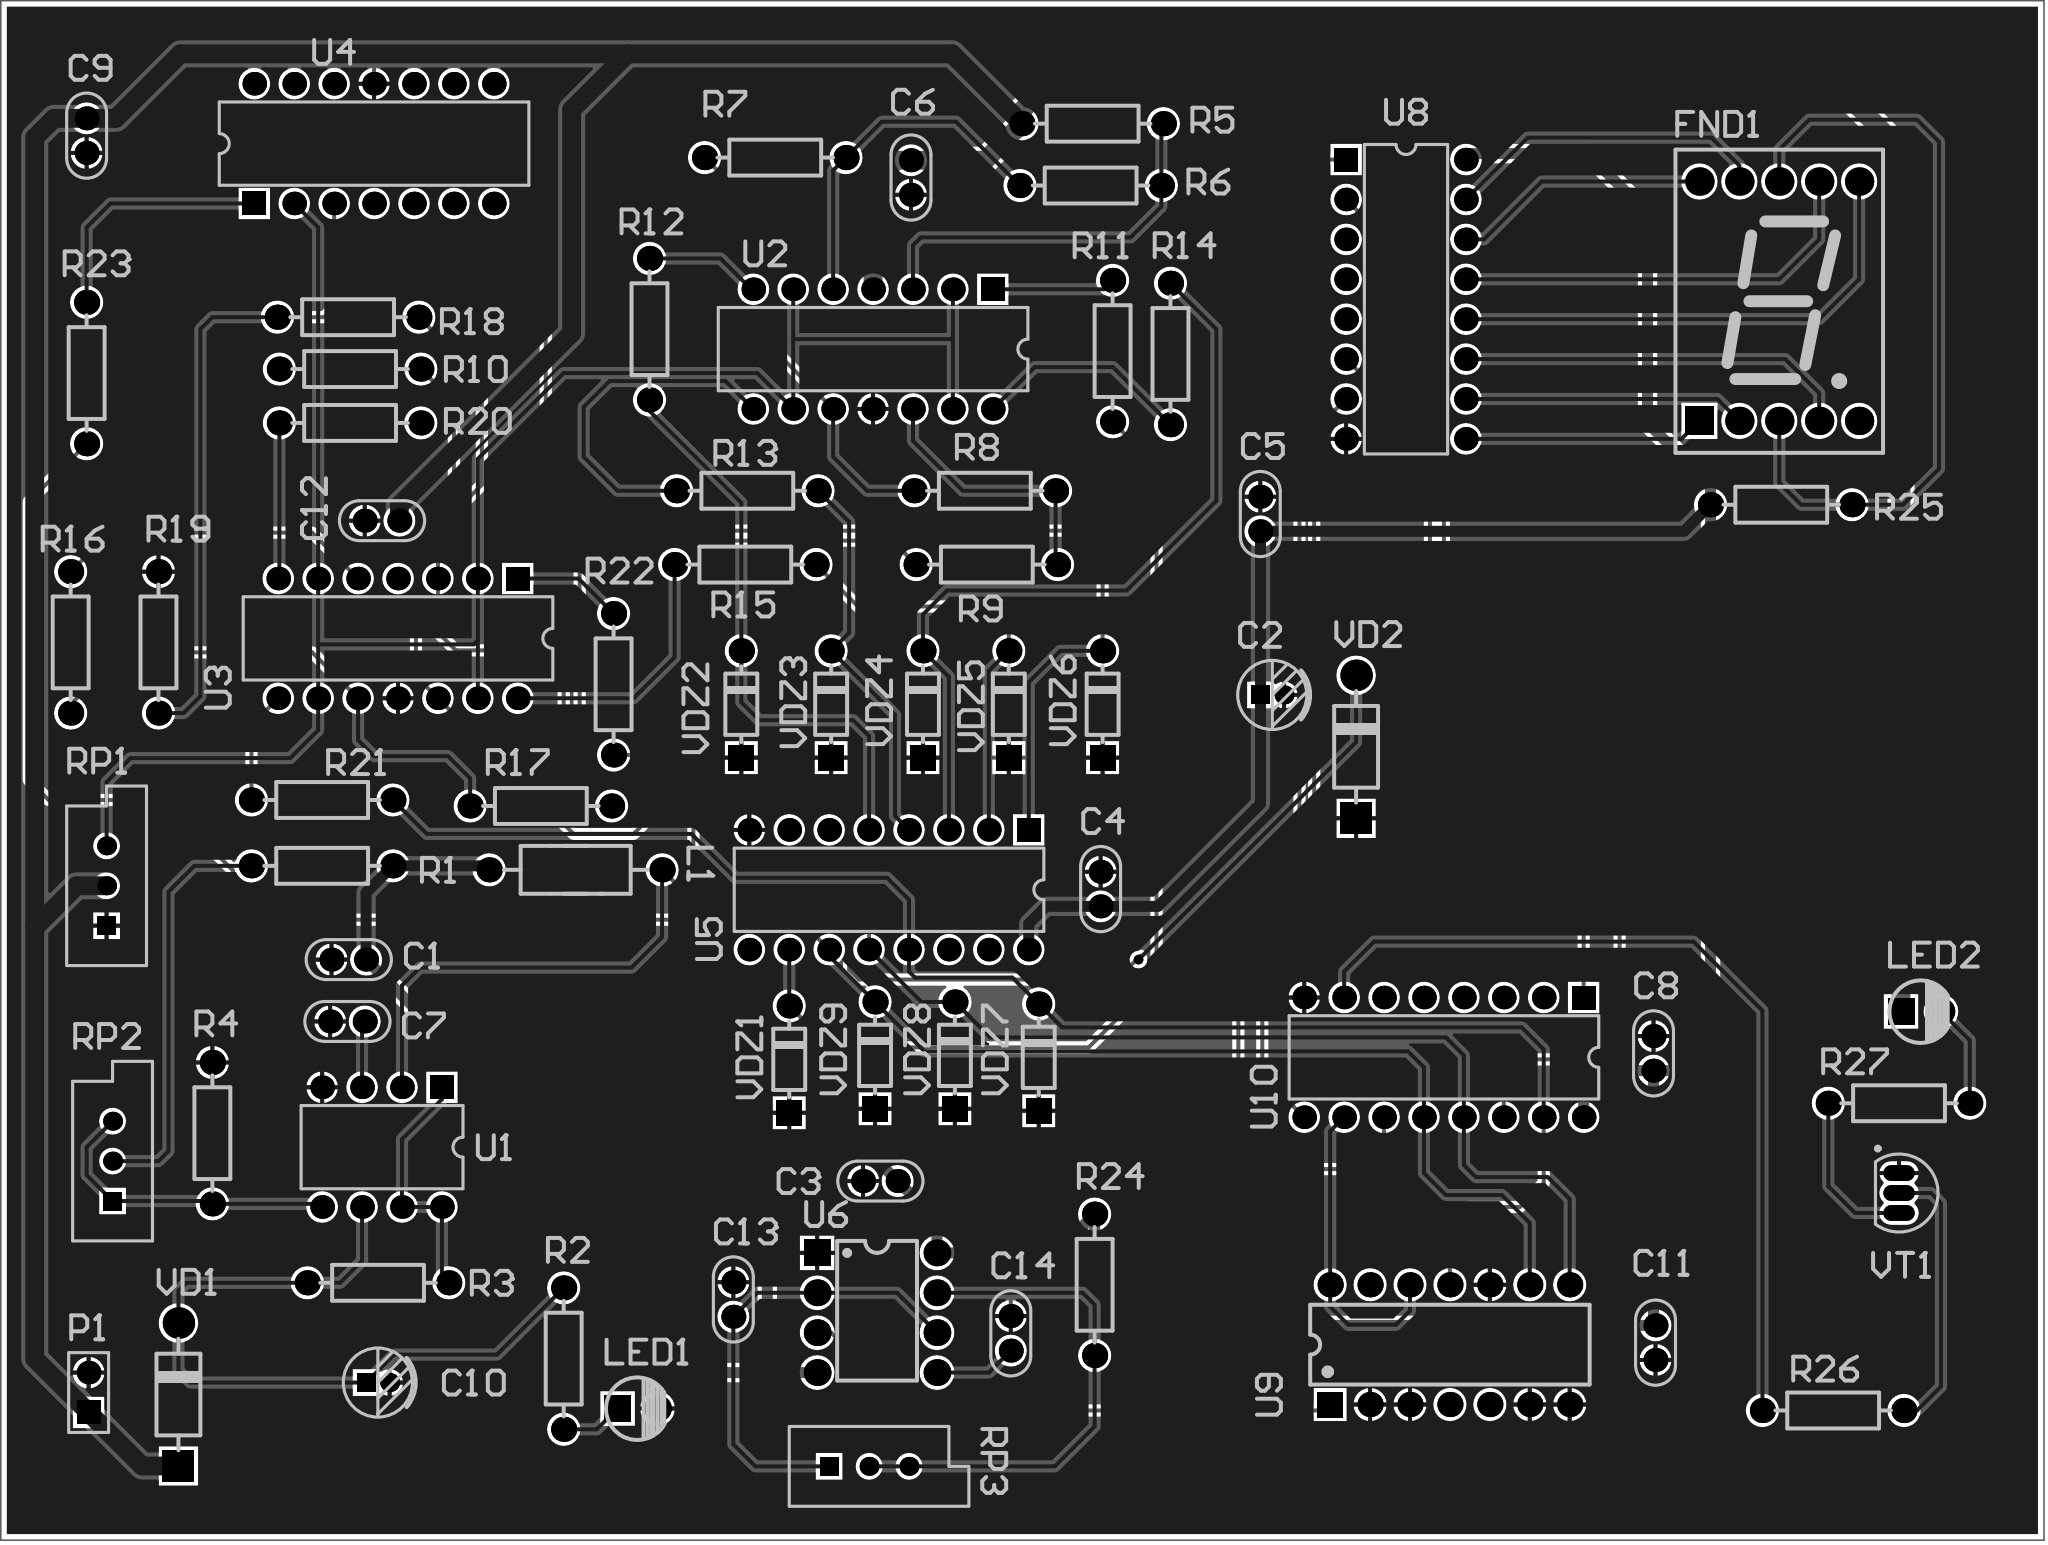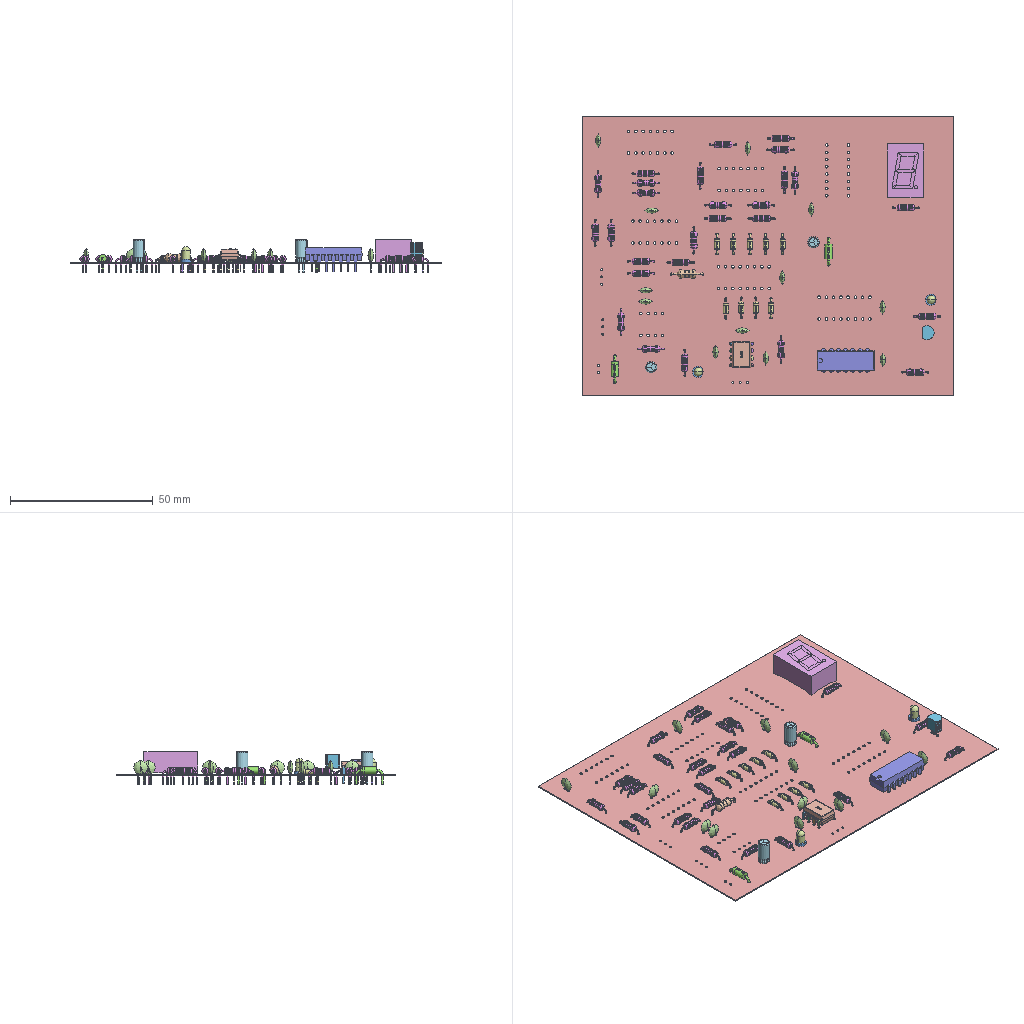Circuit board layout | Altium Designer | box 130 x 98 x 11.6 mm
Layer stack:
# Altium Designer layer stack of  (unit mm; dielectric type: 0 none, 1 core, 2 prepreg, 3 surface material)
index,name,kind,layer,copper_thickness_mm,dielectric_type,dielectric_thickness_mm,dielectric_material,dielectric_constant
0,Top Paste,other,,,,,,
1,Top Overlay,other,,,,,,
2,Top Solder,dielectric,,,3,0.0102,Solder Resist,3.5
3,Top Layer,copper,Top Layer,0.0356,,,,
4,Dielectric 1,dielectric,,,0,0.32,FR-4,4.8
5,Bottom Layer,copper,Bottom Layer,0.0356,,,,
6,Bottom Solder,dielectric,,,3,0.0102,Solder Resist,3.5
7,Bottom Overlay,other,,,,,,
8,Bottom Paste,other,,,,,,
# drill layer pairs: low layer,high layer
drill_pair,Top Layer,Bottom Layer
Part placement:
Designator,Comment,Layer,Footprint,Center-X(mm),Center-Y(mm),Rotation
C1,104,TopLayer,CC_2.2*5,47.541,62.357,180
C2,470UF,TopLayer,CAP_1.5*4*8,106.299,79.205,0
C3,0.1uF,TopLayer,CC_2.2*5,81.364,48.26,180
C4,0.1uF,TopLayer,CC_2.2*5,95.377,66.845,90
C5,0.1uF,TopLayer,CC_2.2*5,105.537,90.721,90
C6,0.1uF,TopLayer,CC_2.2*5,83.312,112.141,270
C7,470PF,TopLayer,CC_2.2*5,47.455,58.42,180
C8,0.1uF,TopLayer,CC_2.2*5,130.556,56.388,90
C9,0.1uF,TopLayer,CC_2.2*5,30.861,114.808,270
C10,100UF,TopLayer,CAP_1.5*4*8,49.391,35.433,360
C11,0.1uF,TopLayer,CC_2.2*5,130.683,37.973,270
C12,0.1uF,TopLayer,CC_2.2*5,49.657,90.297,180
C13,0.1uF,TopLayer,CC_2.2*5,72.009,40.724,90
C14,0.1uF,TopLayer,CC_2.2*5,89.662,38.565,90
FND1,5011B,TopLayer,SMG_0.5-1P,138.557,104.267,0
L1,220uH,TopLayer,AL0307,61.976,68.072,360
LED1,red,TopLayer,LED_3MM-B,65.913,33.782,0
LED2,red,TopLayer,LED_3MM-B,147.574,59.055,0
P1,Header 2,TopLayer,HDR1X2,30.988,34.798,90
R1,3.3K,TopLayer,RS_1/4W,45.847,68.326,360
R2,2.2K,TopLayer,RS_1/4W,61.214,36.957,90
R3,0.5,TopLayer,RS_1/4W,49.403,41.783,180
R4,2.2K,TopLayer,RS_1/4W,38.862,51.308,270
R24,20K,TopLayer,RS_1/4W,94.996,41.656,90
R25,330,TopLayer,RS_1/4W,138.684,91.313,180
R26,4.7K,TopLayer,RS_1/4W,141.986,33.655,180
R27,1K,TopLayer,RS_1/4W,146.177,53.213,360
RP1,100K,TopLayer,VR5,32.131,67.056,90
RP2,5K,TopLayer,VR5,32.512,49.53,90
RP3,50K,TopLayer,VR5,80.645,30.099,360
U1,MC34063AP1,TopLayer,626-05,49.657,50.419,180
U5,SN74LS147N,TopLayer,648-08,81.915,66.802,180
U6,NE555,TopLayer,DIP8,81.153,39.878,0
U8,SN74LS47N,TopLayer,648-08,114.808,104.394,270
U9,SN74LS90,TopLayer,DIP14,117.602,37.846,90
U10,SN74LS85N,TopLayer,648-08,117.221,56.134,180
VD1,1N4007,TopLayer,DO-41,36.703,34.671,90
VD2,1N5819,TopLayer,DO-41,111.633,75.903,90
VT1,TP41,TopLayer,TO-92A,146.177,47.498,180
R5,4.7K,TopLayer,RS_1/4W,94.869,115.57,360
R6,4.7K,TopLayer,RS_1/4W,94.742,111.633,180
R7,4.7K,TopLayer,RS_1/4W,74.676,113.411,180
R8,4.7K,TopLayer,RS_1/4W,88.011,92.202,360
R9,4.7K,TopLayer,RS_1/4W,88.138,87.503,180
R10,4.7K,TopLayer,RS_1/4W,47.625,99.949,180
R11,1K,TopLayer,RS_1/4W,96.139,101.092,270
R12,1K,TopLayer,RS_1/4W,66.675,102.489,270
R13,1K,TopLayer,RS_1/4W,72.898,92.202,360
R14,1K,TopLayer,RS_1/4W,99.822,100.91,90
R15,1K,TopLayer,RS_1/4W,72.771,87.503,360
R16,4.7K,TopLayer,RS_1/4W,29.845,82.55,270
R17,4.7K,TopLayer,RS_1/4W,59.762,72.136,360
R18,4.7K,TopLayer,RS_1/4W,47.498,103.251,180
R19,4.7K,TopLayer,RS_1/4W,35.433,82.55,90
R20,1K,TopLayer,RS_1/4W,47.625,96.52,360
R21,1K,TopLayer,RS_1/4W,45.847,72.517,360
R22,1K,TopLayer,RS_1/4W,64.389,79.883,270
R23,1K,TopLayer,RS_1/4W,30.861,99.695,270
U2,LM324AN,TopLayer,646-06,80.899,101.219,180
U3,LM324AN,TopLayer,646-06,50.673,82.804,180
U4,LM324AN,TopLayer,646-06,49.149,114.3,360
VDZ1,5.1V,TopLayer,DO-35,75.565,56.007,90
VDZ2,5.1V,TopLayer,DO-35,72.517,78.613,90
VDZ3,5.1V,TopLayer,DO-35,78.232,78.613,90
VDZ4,5.1V,TopLayer,DO-35,84.074,78.613,90
VDZ5,5.1V,TopLayer,DO-35,89.535,78.613,90
VDZ6,5.1V,TopLayer,DO-35,95.504,78.613,90
VDZ7,5.1V,TopLayer,DO-35,91.44,56.134,90
VDZ8,5.1V,TopLayer,DO-35,86.106,56.261,90
VDZ9,5.1V,TopLayer,DO-35,81.026,56.261,90
Pad and via stacks:
# Altium Designer via and pad stacks of  (unit mm). Each distinct definition once, with the count of objects using it.
# via: kind,start_layer,end_layer,hole_mm,diameter_mm,mode(0 simple;1 top-mid-bottom;2 full stack),diameter_per_layer,count,example_net
# pad: kind,layer,hole_mm,hole_type(0 round;1 square;2 slot),plating,top_size,top_shape(1 round;2 rect;3 octagon;9 rounded rect),mid_size,bottom_size,mode,footprint,size_per_layer,count,example
pad,Multi-Layer,0.9,0,plated,2x1,1,2x1,2x1,0,TO-92A,,3,VT1.1
pad,Multi-Layer,0.6,0,plated,1.6x1.6,1,1.6x1.6,1.6x1.6,0,RS 1/4W,,54,R26.1
pad,Multi-Layer,0.7,0,plated,1.2x1.2,1,1.2x1.2,1.2x1.2,0,VR5,,6,RP2.3
pad,Multi-Layer,0.7,0,plated,1.2x1.2,2,1.2x1.2,1.2x1.2,0,VR5,,3,RP2.1
pad,Multi-Layer,0.9,0,plated,1.7x1.7,1,1.7x1.7,1.7x1.7,0,LED 3MM-B,,2,LED2.2
pad,Multi-Layer,0.9,0,plated,1.7x1.7,2,1.7x1.7,1.7x1.7,0,LED 3MM-B,,2,LED2.1
pad,Multi-Layer,0.5,0,plated,1.524x1.524,1,1.524x1.524,1.524x1.524,0,CC 2.2*5,,24,C1.1
pad,Multi-Layer,0.6,0,plated,1.2x1.2,2,1.2x1.2,1.2x1.2,0,CAP 1.5*4*8,,2,C2.1
pad,Multi-Layer,0.6,0,plated,1.2x1.2,1,1.2x1.2,1.2x1.2,0,CAP 1.5*4*8,,2,C2.2
pad,Multi-Layer,1,0,plated,2x2,2,2x2,2x2,0,DO-41,,2,VD2.1
pad,Multi-Layer,1,0,plated,2x2,1,2x2,2x2,0,DO-41,,2,VD2.2
pad,Multi-Layer,0.8,0,plated,1.6x1.6,1,1.6x1.6,1.6x1.6,0,AL0307,,2,L1.1
pad,Multi-Layer,0.9,0,plated,1.5x1.5,2,1.5x1.5,1.5x1.5,0,626-05,,1,U1.1
pad,Multi-Layer,0.9,0,plated,1.5x1.5,1,1.5x1.5,1.5x1.5,0,626-05,,7,U1.2
pad,Multi-Layer,0.9,0,plated,1.5x1.5,1,1.5x1.5,1.5x1.5,0,HDR1X2,,1,P1.2
pad,Multi-Layer,0.9,0,plated,1.5x1.5,2,1.5x1.5,1.5x1.5,0,HDR1X2,,1,P1.1
pad,Multi-Layer,0.9,0,plated,1.5x1.5,2,1.5x1.5,1.5x1.5,0,648-08,,3,U5.1
pad,Multi-Layer,0.9,0,plated,1.5x1.5,1,1.5x1.5,1.5x1.5,0,648-08,,45,U5.2
pad,Multi-Layer,0.8,0,plated,1.7x1.7,2,1.7x1.7,1.7x1.7,0,DIP8,,1,U6.1
pad,Multi-Layer,0.8,0,plated,1.7x1.7,1,1.7x1.7,1.7x1.7,0,DIP8,,7,U6.2
pad,Multi-Layer,0.9,0,plated,1.8x1.8,1,1.8x1.8,1.8x1.8,0,SMG 0.5-1P,,9,FND1.10
pad,Multi-Layer,0.9,0,plated,1.8x1.8,2,1.8x1.8,1.8x1.8,0,SMG 0.5-1P,,1,FND1.1
pad,Multi-Layer,0.8128,0,plated,1.6x1.6,2,1.6x1.6,1.6x1.6,0,DIP14,,1,U9.1
pad,Multi-Layer,0.8128,0,plated,1.6x1.6,1,1.6x1.6,1.6x1.6,0,DIP14,,13,U9.2
pad,Multi-Layer,0.8,0,plated,1.6x1.6,2,1.6x1.6,1.6x1.6,0,DO-35,,9,VDZ5.1
pad,Multi-Layer,0.8,0,plated,1.6x1.6,1,1.6x1.6,1.6x1.6,0,DO-35,,9,VDZ5.2
pad,Multi-Layer,0.9,0,plated,1.5x1.5,2,1.5x1.5,1.5x1.5,0,646-06,,3,U4.1
pad,Multi-Layer,0.9,0,plated,1.5x1.5,1,1.5x1.5,1.5x1.5,0,646-06,,39,U4.2
via,Top Layer,Bottom Layer,0.3048,0.6096,0,,1,NetL1_2
Copper pours:
name,layer,net,type(0 solid;1 hatched;2 none)
D,Bottom Layer,GND,0
D,Top Layer,GND,0
Design rules, without the lines most boards share:
# Altium Designer design rules of  (exported by Altium Designer, unit mm)
# columns: name | kind | enabled | priority | scope1 | scope2 | descriptor | typed fields (field=value)
Clearance | 0 | enabled | 1 | All | All | Clearance Constraint (Gap=0.254mm) (All),(All) | gap=0.254
PlaneConnect | 6 | enabled | 1 | All | All | Power Plane Connect Rule(Relief Connect )(Expansion=0.508mm) (Conductor Width=0.254mm) (Air Gap=0.254mm) (Entries=4) (All) | relief_conductor_width=0.254 relief_entries=4 relief_expansion=0.508
PlaneClearance | 12 | enabled | 1 | All | All | Power Plane Clearance (Clearance =0.508mm) (All) | clearance=0.508
PolygonConnect | 20 | enabled | 1 | All | All | Polygon Connect Rule(Relief Connect )(Conductor Width=0.254mm) (Relief Angle=90 Angle) (Entries=4) (Air Gap Width=0.254mm) (All),(All) | connect_style(0=relief,1=direct,2=none)=0 relief_conductor_width=0.254 relief_entries=4
Width | 2 | enabled | 1 | All | All | Width Constraint (Min=0.254mm) (Max=2mm) (Preferred=0.254mm) (All) |
RoutingCorners | 10 | enabled | 1 | All | All | Routing Corners (Style=45-Degree) (Min Setback=2.54mm) (Max Setback=2.54mm) (All) |
RoutingVias | 11 | enabled | 1 | All | All | Routing Via (MinHoleWidth=0.711mm) (MaxHoleWidth=0.711mm) (PreferredHoleWidth=0.711mm) (MinWidth=1.27mm) (MaxWidth=1.27mm) (PreferedWidth=1.27mm) (All) | via_min_hole=0.7112 via_max_hole=0.7112 via_preferred_diameter=1.27 via_preferred_hole=0.7112
PasteMaskExpansion | 14 | enabled | 1 | All | All | Paste Mask Expansion (Expansion =0mm) (All) | expansion=0
SolderMaskExpansion | 13 | enabled | 1 | All | All | Solder Mask Expansion (Expansion =0.102mm) (All) | expansion=0.1016
ComponentClearance | 24 | enabled | 1 | All | All | Component Clearance Constraint ( Horizontal Gap = 0.254mm, Vertical Gap = 0.254mm ) (All),(All)  | gap=0.254
Height | 50 | enabled | 1 | All | All | Height Constraint (Min=0mm) (Max=25.4mm) (Prefered=12.7mm) (All) | min_height=0 max_height=25.4
HoleSize | 42 | enabled | 1 | All | All | Hole Size Constraint (Min=0.025mm) (Max=2.54mm) (All) |
DiffPairsRouting | 51 | enabled | 1 | All | All | Differential Pairs Uncoupled Length using the Gap Constraints (Min=0.254mm) (Max=0.254mm) (Prefered=0.254mm)  and Width Constraints (Min=0.381mm) (Max=0.381mm) (Prefered=0.381mm) (All) |
HoleToHoleClearance | 52 | enabled | 1 | All | All | Hole To Hole Clearance (Gap=0.254mm) (All),(All) | gap=0.254
MinimumSolderMaskSliver | 53 | enabled | 1 | All | All | Minimum Solder Mask Sliver (Gap=0mm) (All),(All) |
SilkToSolderMaskClearance | 54 | enabled | 1 | IsPad | All | Silk To Solder Mask (Clearance=0mm) (IsPad),(All) |
SilkToSilkClearance | 55 | enabled | 1 | All | All | Silk to Silk (Clearance=0mm) (All),(All) |
NetAntennae | 56 | enabled | 1 | All | All | Net Antennae (Tolerance=0mm) (All) |
Classes set for this board:
# Altium Designer classes of  (member kind: 0 net, 1 component, 2 from-to, 3 pad, 4 layer, 5 differential pair, 6 design channel, 7 polygon, 8 structure, 9 xSignal)
# columns: class name | member kind | superclass | members
Sheet1 | 1 | no | C1; C2; C3; C4; C5; C6; C7; C8; C9; C10; C11; C12; C13; C14; FND1; L1; LED1; LED2; P1; R1; R2; R3; R4; R24; R25; R26; R27; RP1; RP2; RP3; U1; U5; U6; U7; U8; U9; U10; VD1; VD2; VT1; R5; R6; R7; R8; R9; R10; R11; R12; R13; R14; R15; R16; R17; R18; R19; R20; R21; R22; R23; U2; U3; U4; VDZ1; VDZ2; VDZ3; VDZ4; VDZ5; VDZ6; VDZ7; VDZ8; VDZ9;